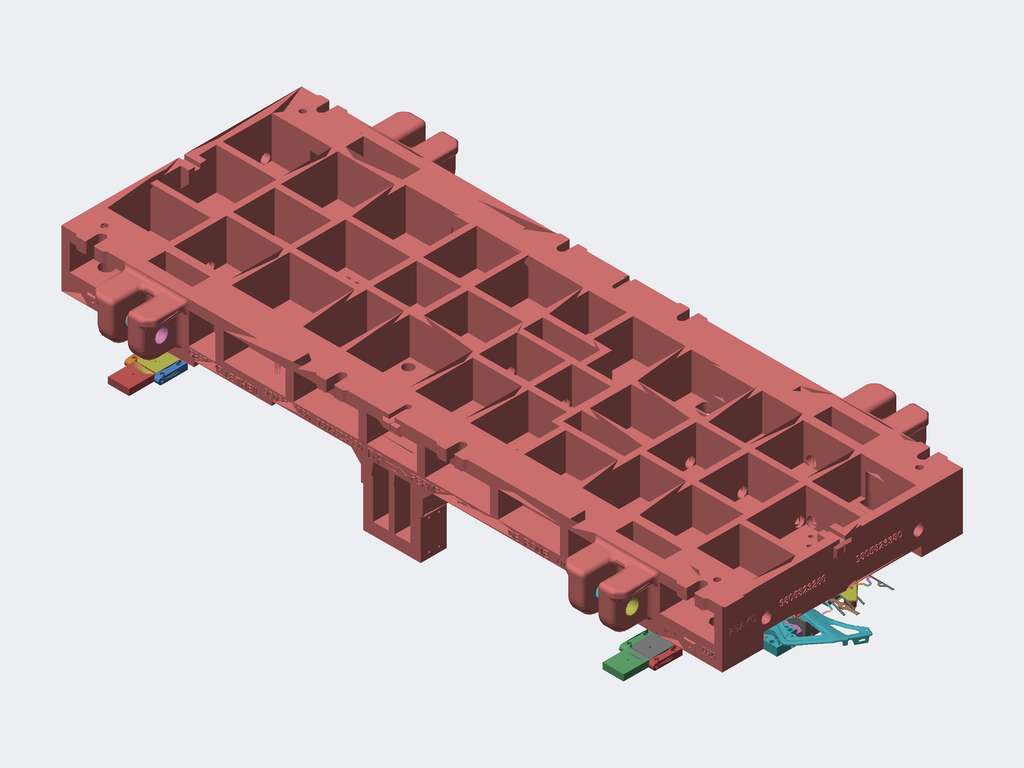Assembly | STEP file | 465 different items | 465 placed
Parts list (item | name | quantity | parent item | size | volume), first 255 of 465 items:
1 | gslz 2016.10.28-13_id1862_x_t | x1 | in gslz 2016.10.28-13_x_t | 105 x 145.1 x 30 mm | 436893 mm3
2 | gslz 2016.10.28-13_id1858_x_t | x1 | in gslz 2016.10.28-13_x_t | 105 x 145.1 x 30 mm | 436893 mm3
3 | gslz 2016.10.28-13_id1854_x_t | x1 | in gslz 2016.10.28-13_x_t | 105 x 145.1 x 30 mm | 436893 mm3
4 | gslz 2016.10.28-13_id1850_x_t | x1 | in gslz 2016.10.28-13_x_t | 105 x 145.1 x 30 mm | 436893 mm3
5 | gslz 2016.10.28-13_id1846_x_t | x1 | in gslz 2016.10.28-13_x_t | 33 x 145.1 x 30 mm | 128184 mm3
6 | gslz 2016.10.28-13_id1842_x_t | x1 | in gslz 2016.10.28-13_x_t | 105 x 145.1 x 30 mm | 436893 mm3
7 | gslz 2016.10.28-13_id1838_x_t | x1 | in gslz 2016.10.28-13_x_t | 105 x 145.1 x 30 mm | 436893 mm3
8 | gslz 2016.10.28-13_id1834_x_t | x1 | in gslz 2016.10.28-13_x_t | 105 x 145.1 x 30 mm | 436893 mm3
9 | gslz 2016.10.28-13_id1830_x_t | x1 | in gslz 2016.10.28-13_x_t | 105 x 145.1 x 30 mm | 436893 mm3
10 | gslz 2016.10.28-13_id1826_x_t | x1 | in gslz 2016.10.28-13_x_t | 23.336 x 25.084 x 18 mm | 4338 mm3
11 | gslz 2016.10.28-13_id1822_x_t | x1 | in gslz 2016.10.28-13_x_t | 23.336 x 25.084 x 18 mm | 4338 mm3
12 | gslz 2016.10.28-13_id1818_x_t | x1 | in gslz 2016.10.28-13_x_t | 78.589 x 55.064 x 12 mm | 30432 mm3
13 | gslz 2016.10.28-13_id1814_x_t | x1 | in gslz 2016.10.28-13_x_t | 79.537 x 58.997 x 10 mm | 15532 mm3
14 | gslz 2016.10.28-13_id1810_x_t | x1 | in gslz 2016.10.28-13_x_t | 101.812 x 70.347 x 10 mm | 22218 mm3
15 | gslz 2016.10.28-13_id1806_x_t | x1 | in gslz 2016.10.28-13_x_t | 101.812 x 70.347 x 10 mm | 22218 mm3
16 | gslz 2016.10.28-13_id1802_x_t | x1 | in gslz 2016.10.28-13_x_t | 30.396 x 23.404 x 12 mm | 3167 mm3
17 | gslz 2016.10.28-13_id1798_x_t | x1 | in gslz 2016.10.28-13_x_t | 30.396 x 23.404 x 12 mm | 3167 mm3
18 | gslz 2016.10.28-13_id1794_x_t | x1 | in gslz 2016.10.28-13_x_t | 48.801 x 30.009 x 15 mm | 3814 mm3
19 | gslz 2016.10.28-13_id1790_x_t | x1 | in gslz 2016.10.28-13_x_t | 48.801 x 30.009 x 15 mm | 3814 mm3
20 | gslz 2016.10.28-13_id1786_x_t | x1 | in gslz 2016.10.28-13_x_t | 29.214 x 38.304 x 56 mm | 22057 mm3
21 | gslz 2016.10.28-13_id1782_x_t | x1 | in gslz 2016.10.28-13_x_t | 37.214 x 54.544 x 22 mm | 10797 mm3
22 | gslz 2016.10.28-13_id1778_x_t | x1 | in gslz 2016.10.28-13_x_t | 41.743 x 29.62 x 14.53 mm | 4507 mm3
23 | gslz 2016.10.28-13_id1774_x_t | x1 | in gslz 2016.10.28-13_x_t | 102.493 x 71.684 x 27.5 mm | 56764 mm3
24 | gslz 2016.10.28-13_id1770_x_t | x1 | in gslz 2016.10.28-13_x_t | 102.493 x 71.684 x 27.5 mm | 56764 mm3
25 | gslz 2016.10.28-13_id1766_x_t | x1 | in gslz 2016.10.28-13_x_t | 159.469 x 183.505 x 86.5 mm | 557397 mm3
26 | gslz 2016.10.28-13_id1762_x_t | x1 | in gslz 2016.10.28-13_x_t | - | -
27 | 9805823280.1BPIECE_SOLIDE_FINALE_id1758_x_t | x1 | in gslz 2016.10.28-13_x_t | 12.56 x 23.021 x 8.234 mm | 240.263 mm3
28 | 1_id1754_x_t | x1 | in gslz 2016.10.28-13_x_t | 45.134 x 45.134 x 19 mm | 11498 mm3
29 | 1_id1750_x_t | x1 | in gslz 2016.10.28-13_x_t | 52.205 x 48.73 x 19 mm | 13276 mm3
30 | gslz 2016.10.28-13_id1746_x_t | x1 | in gslz 2016.10.28-13_x_t | 17 x 26 x 49 mm | 16052 mm3
31 | gslz 2016.10.28-13_id1742_x_t | x1 | in gslz 2016.10.28-13_x_t | 36 x 68 x 6 mm | 13161 mm3
32 | gslz 2016.10.28-13_id1738_x_t | x1 | in gslz 2016.10.28-13_x_t | 36 x 73 x 6 mm | 12869 mm3
33 | gslz 2016.10.28-13_id1734_x_t | x1 | in gslz 2016.10.28-13_x_t | 36 x 68 x 6 mm | 13161 mm3
34 | gslz 2016.10.28-13_id1730_x_t | x1 | in gslz 2016.10.28-13_x_t | 36 x 73 x 6 mm | 12869 mm3
35 | gslz 2016.10.28-13_id1726_x_t | x1 | in gslz 2016.10.28-13_x_t | 45 x 83 x 6 mm | 19739 mm3
36 | gslz 2016.10.28-13_id1722_x_t | x1 | in gslz 2016.10.28-13_x_t | 45 x 88 x 6 mm | 19661 mm3
37 | gslz 2016.10.28-13_id1718_x_t | x1 | in gslz 2016.10.28-13_x_t | 65 x 58 x 6 mm | 19127 mm3
38 | gslz 2016.10.28-13_id1714_x_t | x1 | in gslz 2016.10.28-13_x_t | 65 x 63 x 6 mm | 18675 mm3
39 | gslz 2016.10.28-13_id1710_x_t | x1 | in gslz 2016.10.28-13_x_t | 17 x 25 x 49 mm | 15358 mm3
40 | gslz 2016.10.28-13_id1706_x_t | x1 | in gslz 2016.10.28-13_x_t | 87.307 x 59.069 x 5 mm | 20118 mm3
41 | gslz 2016.10.28-13_id1702_x_t | x1 | in gslz 2016.10.28-13_x_t | 88.351 x 60.113 x 25 mm | 76522 mm3
42 | gslz 2016.10.28-13_id1698_x_t | x1 | in gslz 2016.10.28-13_x_t | 308.791 x 150.802 x 82.369 mm | 1185537 mm3
43 | gslz 2016.10.28-13_id1694_x_t | x1 | in gslz 2016.10.28-13_x_t | 72 x 35 x 5 mm | 11553 mm3
44 | gslz 2016.10.28-13_id1690_x_t | x1 | in gslz 2016.10.28-13_x_t | 69.906 x 50.319 x 5 mm | 9493 mm3
45 | gslz 2016.10.28-13_id1686_x_t | x1 | in gslz 2016.10.28-13_x_t | 64.831 x 66.474 x 5 mm | 11193 mm3
46 | gslz 2016.10.28-13_id1682_x_t | x1 | in gslz 2016.10.28-13_x_t | 67.358 x 53.937 x 5 mm | 9493 mm3
47 | gslz 2016.10.28-13_id1678_x_t | x1 | in gslz 2016.10.28-13_x_t | 73 x 36 x 26 mm | 45297 mm3
48 | gslz 2016.10.28-13_id1674_x_t | x1 | in gslz 2016.10.28-13_x_t | 70.882 x 51.053 x 36 mm | 51884 mm3
49 | gslz 2016.10.28-13_id1670_x_t | x1 | in gslz 2016.10.28-13_x_t | 68.435 x 55.014 x 26 mm | 39925 mm3
50 | gslz 2016.10.28-13_id1666_x_t | x1 | in gslz 2016.10.28-13_x_t | 65.839 x 67.482 x 31 mm | 54828 mm3
51 | gslz 2016.10.28-13_id1662_x_t | x1 | in gslz 2016.10.28-13_x_t | 29.227 x 19.541 x 70.5 mm | 21986 mm3
52 | gslz 2016.10.28-13_id1658_x_t | x1 | in gslz 2016.10.28-13_x_t | 32.149 x 22.13 x 70 mm | 26166 mm3
53 | gslz 2016.10.28-13_id1654_x_t | x1 | in gslz 2016.10.28-13_x_t | 46 x 23 x 10 mm | 9308 mm3
54 | gslz 2016.10.28-13_id1650_x_t | x1 | in gslz 2016.10.28-13_x_t | 43.888 x 21.981 x 24.856 mm | 5888 mm3
55 | gslz 2016.10.28-13_id1646_x_t | x1 | in gslz 2016.10.28-13_x_t | 105 x 520 x 15 mm | 667550 mm3
56 | gslz 2016.10.28-13_id1642_x_t | x1 | in gslz 2016.10.28-13_x_t | 180 x 40 x 32 mm | 197761 mm3
57 | gslz 2016.10.28-13_id1638_x_t | x1 | in gslz 2016.10.28-13_x_t | 110 x 90.115 x 79.8 mm | 541473 mm3
58 | gslz 2016.10.28-13_id1634_x_t | x1 | in gslz 2016.10.28-13_x_t | 39.238 x 33.552 x 28.984 mm | 15189 mm3
59 | gslz 2016.10.28-13_id1630_x_t | x1 | in gslz 2016.10.28-13_x_t | 158 x 98 x 72.916 mm | 768512 mm3
60 | gslz 2016.10.28-13_id1626_x_t | x1 | in gslz 2016.10.28-13_x_t | 42.516 x 42.404 x 26.831 mm | 17674 mm3
61 | gslz 2016.10.28-13_id1622_x_t | x1 | in gslz 2016.10.28-13_x_t | 17 x 20 x 49 mm | 11659 mm3
62 | gslz 2016.10.28-13_id1618_x_t | x1 | in gslz 2016.10.28-13_x_t | 57 x 88 x 63 mm | 168012 mm3
63 | 9805823380.1BPIECE_SOLIDE_FINALE_id1614_x_t | x1 | in gslz 2016.10.28-13_x_t | 252.902 x 148 x 67.965 mm | 1153711 mm3
64 | gslz 2016.10.28-13_id1610_x_t | x1 | in gslz 2016.10.28-13_x_t | 85 x 71 x 16 mm | 81626 mm3
65 | gslz 2016.10.28-13_id1606_x_t | x1 | in gslz 2016.10.28-13_x_t | 85 x 71 x 32 mm | 153487 mm3
66 | gslz 2016.10.28-13_id1602_x_t | x1 | in gslz 2016.10.28-13_x_t | 85 x 28 x 6 mm | 11529 mm3
67 | gslz 2016.10.28-13_id1598_x_t | x1 | in gslz 2016.10.28-13_x_t | 85 x 33 x 6 mm | 12707 mm3
68 | gslz 2016.10.28-13_id1594_x_t | x1 | in gslz 2016.10.28-13_x_t | 135 x 28 x 6 mm | 19929 mm3
69 | gslz 2016.10.28-13_id1590_x_t | x1 | in gslz 2016.10.28-13_x_t | 135 x 33 x 6 mm | 22607 mm3
70 | gslz 2016.10.28-13_id1586_x_t | x1 | in gslz 2016.10.28-13_x_t | 76 x 28 x 6 mm | 11241 mm3
71 | gslz 2016.10.28-13_id1582_x_t | x1 | in gslz 2016.10.28-13_x_t | 76 x 33 x 6 mm | 12149 mm3
72 | gslz 2016.10.28-13_id1578_x_t | x1 | in gslz 2016.10.28-13_x_t | 150 x 28 x 6 mm | 23673 mm3
73 | gslz 2016.10.28-13_id1574_x_t | x1 | in gslz 2016.10.28-13_x_t | 150 x 33 x 6 mm | 26801 mm3
74 | gslz 2016.10.28-13_id1570_x_t | x1 | in gslz 2016.10.28-13_x_t | 730 x 120 x 32 mm | 1766877 mm3
75 | gslz 2016.10.28-13_id1566_x_t | x1 | in gslz 2016.10.28-13_x_t | 810 x 120 x 32 mm | 2005033 mm3
76 | gslz 2016.10.28-13_id1562_x_t | x1 | in gslz 2016.10.28-13_x_t | 27.764 x 27.764 x 29.737 mm | 5874 mm3
77 | gslz 2016.10.28-13_id1558_x_t | x1 | in gslz 2016.10.28-13_x_t | 124.158 x 124.158 x 39.786 mm | 35566 mm3
78 | gslz 2016.10.28-13_id1554_x_t | x1 | in gslz 2016.10.28-13_x_t | 124.158 x 124.158 x 39.786 mm | 35566 mm3
79 | gslz 2016.10.28-13_id1550_x_t | x1 | in gslz 2016.10.28-13_x_t | 124.501 x 121.928 x 56.838 mm | 87407 mm3
80 | gslz 2016.10.28-13_id1546_x_t | x1 | in gslz 2016.10.28-13_x_t | 121.928 x 124.501 x 56.838 mm | 87407 mm3
81 | gslz 2016.10.28-13_id1542_x_t | x1 | in gslz 2016.10.28-13_x_t | 234.759 x 255.973 x 69 mm | 1431737 mm3
82 | gslz 2016.10.28-13_id1538_x_t | x1 | in gslz 2016.10.28-13_x_t | 27.148 x 27.148 x 16.361 mm | 2153 mm3
83 | gslz 2016.10.28-13_id1534_x_t | x1 | in gslz 2016.10.28-13_x_t | 27.622 x 23.712 x 48.072 mm | 19234 mm3
84 | gslz 2016.10.28-13_id1530_x_t | x1 | in gslz 2016.10.28-13_x_t | 123 x 53 x 40 mm | 161709 mm3
85 | gslz 2016.10.28-13_id1526_x_t | x1 | in gslz 2016.10.28-13_x_t | 45 x 30 x 75.242 mm | 77989 mm3
86 | gslz 2016.10.28-13_id1522_x_t | x1 | in gslz 2016.10.28-13_x_t | - | 122117 mm3
87 | gslz 2016.10.28-13_id1518_x_t | x1 | in gslz 2016.10.28-13_x_t | 29.762 x 31.599 x 21.259 mm | 4382 mm3
88 | gslz 2016.10.28-13_id1514_x_t | x1 | in gslz 2016.10.28-13_x_t | 198.697 x 124.174 x 92.051 mm | 929934 mm3
89 | gslz 2016.10.28-13_id1510_x_t | x1 | in gslz 2016.10.28-13_x_t | 60.365 x 38.336 x 39 mm | 43186 mm3
90 | gslz 2016.10.28-13_id1506_x_t | x1 | in gslz 2016.10.28-13_x_t | 44.234 x 36.078 x 44 mm | 40757 mm3
91 | gslz 2016.10.28-13_id1502_x_t | x1 | in gslz 2016.10.28-13_x_t | - | -
92 | gslz 2016.10.28-13_id1498_x_t | x1 | in gslz 2016.10.28-13_x_t | - | -
93 | gslz 2016.10.28-13_id1494_x_t | x1 | in gslz 2016.10.28-13_x_t | - | -
94 | gslz 2016.10.28-13_id1490_x_t | x1 | in gslz 2016.10.28-13_x_t | - | -
95 | gslz 2016.10.28-13_id1486_x_t | x1 | in gslz 2016.10.28-13_x_t | - | -
96 | gslz 2016.10.28-13_id1482_x_t | x1 | in gslz 2016.10.28-13_x_t | 48.587 x 48.391 x 29.021 mm | 10993 mm3
97 | gslz 2016.10.28-13_id1478_x_t | x1 | in gslz 2016.10.28-13_x_t | 25.456 x 25.456 x 27 mm | 6738 mm3
98 | gslz 2016.10.28-13_id1474_x_t | x1 | in gslz 2016.10.28-13_x_t | 22.953 x 24.888 x 27 mm | 6892 mm3
99 | gslz 2016.10.28-13_id1470_x_t | x1 | in gslz 2016.10.28-13_x_t | 66.885 x 98.566 x 27.5 mm | 53451 mm3
100 | gslz 2016.10.28-13_id1466_x_t | x1 | in gslz 2016.10.28-13_x_t | 67.638 x 102.464 x 10 mm | 22218 mm3
101 | gslz 2016.10.28-13_id1462_x_t | x1 | in gslz 2016.10.28-13_x_t | 67.638 x 102.464 x 10 mm | 22218 mm3
102 | gslz 2016.10.28-13_id1458_x_t | x1 | in gslz 2016.10.28-13_x_t | 66.885 x 98.566 x 27.5 mm | 53451 mm3
103 | gslz 2016.10.28-13_id1454_x_t | x1 | in gslz 2016.10.28-13_x_t | 81.802 x 53.748 x 52 mm | 84086 mm3
104 | gslz 2016.10.28-13_id1450_x_t | x1 | in gslz 2016.10.28-13_x_t | 160.575 x 107.178 x 72.851 mm | 541622 mm3
105 | gslz 2016.10.28-13_id1446_x_t | x1 | in gslz 2016.10.28-13_x_t | 9.039 x 11.595 x 1.56 mm | 84.551 mm3
106 | gslz 2016.10.28-13_id1442_x_t | x1 | in gslz 2016.10.28-13_x_t | - | -
107 | gslz 2016.10.28-13_id1438_x_t | x1 | in gslz 2016.10.28-13_x_t | - | -
108 | gslz 2016.10.28-13_id1434_x_t | x1 | in gslz 2016.10.28-13_x_t | - | -
109 | gslz 2016.10.28-13_id1430_x_t | x1 | in gslz 2016.10.28-13_x_t | - | -
110 | gslz 2016.10.28-13_id1426_x_t | x1 | in gslz 2016.10.28-13_x_t | - | -
111 | gslz 2016.10.28-13_id1422_x_t | x1 | in gslz 2016.10.28-13_x_t | 96.313 x 39.023 x 74.019 mm | 168785 mm3
112 | gslz 2016.10.28-13_id1418_x_t | x1 | in gslz 2016.10.28-13_x_t | 415 x 296 x 77.793 mm | 6493168 mm3
113 | gslz 2016.10.28-13_id1414_x_t | x1 | in gslz 2016.10.28-13_x_t | - | -
114 | gslz 2016.10.28-13_id1410_x_t | x1 | in gslz 2016.10.28-13_x_t | - | -
115 | gslz 2016.10.28-13_id1406_x_t | x1 | in gslz 2016.10.28-13_x_t | - | -
116 | gslz 2016.10.28-13_id1402_x_t | x1 | in gslz 2016.10.28-13_x_t | 90.51 x 90.51 x 10 mm | 22218 mm3
117 | gslz 2016.10.28-13_id1398_x_t | x1 | in gslz 2016.10.28-13_x_t | 90.51 x 90.51 x 10 mm | 22218 mm3
118 | gslz 2016.10.28-13_id1394_x_t | x1 | in gslz 2016.10.28-13_x_t | 50.205 x 48.083 x 16 mm | 10037 mm3
119 | gslz 2016.10.28-13_id1390_x_t | x1 | in gslz 2016.10.28-13_x_t | 37.477 x 39.598 x 16 mm | 7157 mm3
120 | gslz 2016.10.28-13_id1386_x_t | x1 | in gslz 2016.10.28-13_x_t | 91.57 x 91.57 x 27.5 mm | 56764 mm3
121 | gslz 2016.10.28-13_id1382_x_t | x1 | in gslz 2016.10.28-13_x_t | 43.55 x 43.55 x 48.008 mm | 15438 mm3
122 | gslz 2016.10.28-13_id1378_x_t | x1 | in gslz 2016.10.28-13_x_t | 91.57 x 91.57 x 27.5 mm | 56764 mm3
123 | gslz 2016.10.28-13_id1374_x_t | x1 | in gslz 2016.10.28-13_x_t | 48.79 x 48.79 x 60 mm | 42680 mm3
124 | gslz 2016.10.28-13_id1370_x_t | x1 | in gslz 2016.10.28-13_x_t | 46.5 x 32.8 x 73 mm | 100113 mm3
125 | gslz 2016.10.28-13_id1366_x_t | x1 | in gslz 2016.10.28-13_x_t | 51.5 x 24.8 x 73 mm | 72067 mm3
126 | gslz 2016.10.28-13_id1362_x_t | x1 | in gslz 2016.10.28-13_x_t | - | -
127 | gslz 2016.10.28-13_id1358_x_t | x1 | in gslz 2016.10.28-13_x_t | 114 x 26.5 x 48 mm | 106202 mm3
128 | gslz 2016.10.28-13_id1354_x_t | x1 | in gslz 2016.10.28-13_x_t | 73.861 x 76.347 x 57.728 mm | 171700 mm3
129 | gslz 2016.10.28-13_id1350_x_t | x1 | in gslz 2016.10.28-13_x_t | 339.5 x 207 x 81.123 mm | 2655764 mm3
130 | gslz 2016.10.28-13_id1346_x_t | x1 | in gslz 2016.10.28-13_x_t | - | -
131 | gslz 2016.10.28-13_id1342_x_t | x1 | in gslz 2016.10.28-13_x_t | 347 x 40 x 48 mm | 605773 mm3
132 | gslz 2016.10.28-13_id1338_x_t | x1 | in gslz 2016.10.28-13_x_t | 348 x 40 x 48 mm | 621204 mm3
133 | gslz 2016.10.28-13_id1334_x_t | x1 | in gslz 2016.10.28-13_x_t | 95 x 65 x 32 mm | 157873 mm3
134 | gslz 2016.10.28-13_id1330_x_t | x1 | in gslz 2016.10.28-13_x_t | 12.175 x 9.008 x 2.356 mm | 107.013 mm3
135 | gslz 2016.10.28-13_id1326_x_t | x1 | in gslz 2016.10.28-13_x_t | 8.284 x 8.42 x 2.147 mm | 67.466 mm3
136 | FINAL_SOLID_PART_id1322_x_t | x1 | in gslz 2016.10.28-13_x_t | - | -
137 | gslz 2016.10.28-13_id1318_x_t | x1 | in gslz 2016.10.28-13_x_t | 117.473 x 52.739 x 8.208 mm | 4131 mm3
138 | gslz 2016.10.28-13_id1314_x_t | x1 | in gslz 2016.10.28-13_x_t | - | -
139 | gslz 2016.10.28-13_id1310_x_t | x1 | in gslz 2016.10.28-13_x_t | - | -
140 | gslz 2016.10.28-13_id1306_x_t | x1 | in gslz 2016.10.28-13_x_t | - | -
141 | gslz 2016.10.28-13_id1302_x_t | x1 | in gslz 2016.10.28-13_x_t | - | -
142 | gslz 2016.10.28-13_id1298_x_t | x1 | in gslz 2016.10.28-13_x_t | - | -
143 | gslz 2016.10.28-13_id1294_x_t | x1 | in gslz 2016.10.28-13_x_t | - | -
144 | gslz 2016.10.28-13_id1290_x_t | x1 | in gslz 2016.10.28-13_x_t | - | -
145 | gslz 2016.10.28-13_id1286_x_t | x1 | in gslz 2016.10.28-13_x_t | - | -
146 | gslz 2016.10.28-13_id1282_x_t | x1 | in gslz 2016.10.28-13_x_t | - | -
147 | gslz 2016.10.28-13_id1278_x_t | x1 | in gslz 2016.10.28-13_x_t | - | -
148 | gslz 2016.10.28-13_id1274_x_t | x1 | in gslz 2016.10.28-13_x_t | - | -
149 | gslz 2016.10.28-13_id1270_x_t | x1 | in gslz 2016.10.28-13_x_t | - | -
150 | gslz 2016.10.28-13_id1266_x_t | x1 | in gslz 2016.10.28-13_x_t | - | -
151 | gslz 2016.10.28-13_id1262_x_t | x1 | in gslz 2016.10.28-13_x_t | - | -
152 | gslz 2016.10.28-13_id1258_x_t | x1 | in gslz 2016.10.28-13_x_t | - | 526.34 mm3
153 | gslz 2016.10.28-13_id1254_x_t | x1 | in gslz 2016.10.28-13_x_t | 50.336 x 46.733 x 12.552 mm | 985.225 mm3
154 | gslz 2016.10.28-13_id1250_x_t | x1 | in gslz 2016.10.28-13_x_t | 40.597 x 86.839 x 25.215 mm | 1239 mm3
155 | gslz 2016.10.28-13_id1246_x_t | x1 | in gslz 2016.10.28-13_x_t | - | -
156 | gslz 2016.10.28-13_id1242_x_t | x1 | in gslz 2016.10.28-13_x_t | - | -
157 | gslz 2016.10.28-13_id1238_x_t | x1 | in gslz 2016.10.28-13_x_t | - | -
158 | gslz 2016.10.28-13_id1234_x_t | x1 | in gslz 2016.10.28-13_x_t | - | -
159 | gslz 2016.10.28-13_id1230_x_t | x1 | in gslz 2016.10.28-13_x_t | 63.363 x 44.787 x 14.43 mm | 927.066 mm3
160 | gslz 2016.10.28-13_id1226_x_t | x1 | in gslz 2016.10.28-13_x_t | - | 746.006 mm3
161 | gslz 2016.10.28-13_id1222_x_t | x1 | in gslz 2016.10.28-13_x_t | - | 746.006 mm3
162 | gslz 2016.10.28-13_id1218_x_t | x1 | in gslz 2016.10.28-13_x_t | 63.363 x 44.787 x 14.43 mm | 927.564 mm3
163 | gslz 2016.10.28-13_id1214_x_t | x1 | in gslz 2016.10.28-13_x_t | 335 x 25.5 x 4 mm | 5252 mm3
164 | gslz 2016.10.28-13_id1210_x_t | x1 | in gslz 2016.10.28-13_x_t | 335 x 25.5 x 4 mm | 5252 mm3
165 | gslz 2016.10.28-13_id1206_x_t | x1 | in gslz 2016.10.28-13_x_t | 335 x 25.5 x 4 mm | 5252 mm3
166 | gslz 2016.10.28-13_id1202_x_t | x1 | in gslz 2016.10.28-13_x_t | 335 x 25.5 x 4 mm | 5252 mm3
167 | gslz 2016.10.28-13_id1198_x_t | x1 | in gslz 2016.10.28-13_x_t | 235 x 25.5 x 4 mm | 3805 mm3
168 | FINAL_SOLID_PART_id1194_x_t | x1 | in gslz 2016.10.28-13_x_t | - | -
169 | FINAL_SOLID_PART_id1190_x_t | x1 | in gslz 2016.10.28-13_x_t | - | -
170 | gslz 2016.10.28-13_id1186_x_t | x1 | in gslz 2016.10.28-13_x_t | - | -
171 | gslz 2016.10.28-13_id1182_x_t | x1 | in gslz 2016.10.28-13_x_t | - | -
172 | gslz 2016.10.28-13_id1178_x_t | x1 | in gslz 2016.10.28-13_x_t | 12.2 x 12.2 x 1.25 mm | 146.123 mm3
173 | gslz 2016.10.28-13_id1174_x_t | x1 | in gslz 2016.10.28-13_x_t | 40 x 20 x 1.25 mm | 719.671 mm3
174 | gslz 2016.10.28-13_id1170_x_t | x1 | in gslz 2016.10.28-13_x_t | 6.934 x 8.042 x 1.25 mm | 0.6004 mm3
175 | gslz 2016.10.28-13_id1166_x_t | x1 | in gslz 2016.10.28-13_x_t | 216.271 x 15 x 1.25 mm | 4055 mm3
176 | gslz 2016.10.28-13_id1162_x_t | x1 | in gslz 2016.10.28-13_x_t | 8.449 x 8.449 x 1.25 mm | 67.248 mm3
177 | gslz 2016.10.28-13_id1158_x_t | x1 | in gslz 2016.10.28-13_x_t | 12.076 x 9.187 x 1.25 mm | 107.013 mm3
178 | gslz 2016.10.28-13_id1154_x_t | x1 | in gslz 2016.10.28-13_x_t | 8.449 x 8.449 x 1.25 mm | 67.248 mm3
179 | gslz 2016.10.28-13_id1150_x_t | x1 | in gslz 2016.10.28-13_x_t | 12.076 x 9.187 x 1.25 mm | 107.013 mm3
180 | gslz 2016.10.28-13_id1146_x_t | x1 | in gslz 2016.10.28-13_x_t | 159.005 x 29 x 8 mm | 3787 mm3
181 | gslz 2016.10.28-13_id1142_x_t | x1 | in gslz 2016.10.28-13_x_t | 335 x 29 x 8 mm | 7083 mm3
182 | gslz 2016.10.28-13_id1138_x_t | x1 | in gslz 2016.10.28-13_x_t | 335 x 29 x 8 mm | 7083 mm3
183 | gslz 2016.10.28-13_id1134_x_t | x1 | in gslz 2016.10.28-13_x_t | 335 x 29 x 8 mm | 7083 mm3
184 | gslz 2016.10.28-13_id1130_x_t | x1 | in gslz 2016.10.28-13_x_t | 335 x 29 x 8 mm | 7083 mm3
185 | 9805823380.1BPIECE_SOLIDE_FINALE_id1126_x_t | x1 | in gslz 2016.10.28-13_x_t | 308.018 x 147.7 x 55.936 mm | 34010 mm3
186 | gslz 2016.10.28-13_id1122_x_t | x1 | in gslz 2016.10.28-13_x_t | 139 x 100 x 32 mm | 383578 mm3
187 | gslz 2016.10.28-13_id1118_x_t | x1 | in gslz 2016.10.28-13_x_t | 335 x 29 x 8 mm | 7083 mm3
188 | gslz 2016.10.28-13_id1114_x_t | x1 | in gslz 2016.10.28-13_x_t | 6.882 x 6.913 x 8.538 mm | 70.931 mm3
189 | gslz 2016.10.28-13_id1110_x_t | x1 | in gslz 2016.10.28-13_x_t | 9.039 x 11.595 x 1.56 mm | 84.551 mm3
190 | gslz 2016.10.28-13_id1106_x_t | x1 | in gslz 2016.10.28-13_x_t | 8.332 x 8.174 x 3.149 mm | 67.466 mm3
191 | gslz 2016.10.28-13_id1102_x_t | x1 | in gslz 2016.10.28-13_x_t | 12.193 x 8.988 x 2.236 mm | 107.013 mm3
192 | gslz 2016.10.28-13_id1098_x_t | x1 | in gslz 2016.10.28-13_x_t | 117.479 x 52.908 x 8.668 mm | 4131 mm3
193 | gslz 2016.10.28-13_id1094_x_t | x1 | in gslz 2016.10.28-13_x_t | 18.724 x 18.722 x 8.278 mm | 240.264 mm3
194 | gslz 2016.10.28-13_id1090_x_t | x1 | in gslz 2016.10.28-13_x_t | 18.265 x 18.776 x 11.14 mm | 240.265 mm3
195 | gslz 2016.10.28-13_id1086_x_t | x1 | in gslz 2016.10.28-13_x_t | 6.311 x 6.312 x 2.41 mm | 37.737 mm3
196 | gslz 2016.10.28-13_id1082_x_t | x1 | in gslz 2016.10.28-13_x_t | 11.029 x 10.034 x 2.548 mm | 84.369 mm3
197 | gslz 2016.10.28-13_id1078_x_t | x1 | in gslz 2016.10.28-13_x_t | 8.197 x 8.356 x 2.88 mm | 67.248 mm3
198 | gslz 2016.10.28-13_id1074_x_t | x1 | in gslz 2016.10.28-13_x_t | 12.113 x 9.24 x 3.468 mm | 107.013 mm3
199 | gslz 2016.10.28-13_id1070_x_t | x1 | in gslz 2016.10.28-13_x_t | 10.965 x 9.974 x 2.304 mm | 84.369 mm3
200 | gslz 2016.10.28-13_id1066_x_t | x1 | in gslz 2016.10.28-13_x_t | 6.254 x 6.275 x 1.796 mm | 37.737 mm3
201 | gslz 2016.10.28-13_id1062_x_t | x1 | in gslz 2016.10.28-13_x_t | 6.872 x 6.937 x 8.903 mm | 72.493 mm3
202 | gslz 2016.10.28-13_id1058_x_t | x1 | in gslz 2016.10.28-13_x_t | 12.113 x 9.24 x 3.468 mm | 107.013 mm3
203 | gslz 2016.10.28-13_id1054_x_t | x1 | in gslz 2016.10.28-13_x_t | 6.254 x 6.275 x 1.796 mm | 37.737 mm3
204 | gslz 2016.10.28-13_id1050_x_t | x1 | in gslz 2016.10.28-13_x_t | 10.965 x 9.974 x 2.304 mm | 84.369 mm3
205 | gslz 2016.10.28-13_id1046_x_t | x1 | in gslz 2016.10.28-13_x_t | 8.197 x 8.356 x 2.88 mm | 67.248 mm3
206 | 9805823380.1BPIECE_SOLIDE_FINALE_id1042_x_t | x1 | in gslz 2016.10.28-13_x_t | 329.111 x 160.705 x 37.841 mm | 35454 mm3
207 | gslz 2016.10.28-13_id1038_x_t | x1 | in gslz 2016.10.28-13_x_t | 335 x 25.5 x 4 mm | 5252 mm3
208 | gslz 2016.10.28-13_id1034_x_t | x1 | in gslz 2016.10.28-13_x_t | 253.449 x 25.5 x 4 mm | 4072 mm3
209 | gslz 2016.10.28-13_id1030_x_t | x1 | in gslz 2016.10.28-13_x_t | 335 x 25.5 x 4 mm | 5252 mm3
210 | gslz 2016.10.28-13_id1026_x_t | x1 | in gslz 2016.10.28-13_x_t | 335 x 25.5 x 4 mm | 5252 mm3
211 | gslz 2016.10.28-13_id1022_x_t | x1 | in gslz 2016.10.28-13_x_t | 335 x 25.5 x 4 mm | 5252 mm3
212 | gslz 2016.10.28-13_id1018_x_t | x1 | in gslz 2016.10.28-13_x_t | 335 x 25.5 x 4 mm | 5252 mm3
213 | gslz 2016.10.28-13_id1014_x_t | x1 | in gslz 2016.10.28-13_x_t | 335 x 25.5 x 4 mm | 5252 mm3
214 | gslz 2016.10.28-13_id1010_x_t | x1 | in gslz 2016.10.28-13_x_t | 12.3 x 12.3 x 1.25 mm | 148.529 mm3
215 | gslz 2016.10.28-13_id1006_x_t | x1 | in gslz 2016.10.28-13_x_t | 12.3 x 12.3 x 1.25 mm | 148.529 mm3
216 | 9805823380.1BPIECE_SOLIDE_FINALE_id1002_x_t | x1 | in gslz 2016.10.28-13_x_t | 307.193 x 147.409 x 65.496 mm | 34010 mm3
217 | 9805823380.1BPIECE_SOLIDE_FINALE_id998_x_t | x1 | in gslz 2016.10.28-13_x_t | 307.193 x 147.409 x 65.496 mm | 34012 mm3
218 | gslz 2016.10.28-13_id994_x_t | x1 | in gslz 2016.10.28-13_x_t | 903 x 64 x 38 mm | 1224228 mm3
219 | gslz 2016.10.28-13_id990_x_t | x1 | in gslz 2016.10.28-13_x_t | 730 x 68 x 38 mm | 1131774 mm3
220 | gslz 2016.10.28-13_id986_x_t | x1 | in gslz 2016.10.28-13_x_t | 117.479 x 52.908 x 8.668 mm | 4131 mm3
221 | gslz 2016.10.28-13_id982_x_t | x1 | in gslz 2016.10.28-13_x_t | - | -
222 | FINAL_SOLID_PART_id978_x_t | x1 | in gslz 2016.10.28-13_x_t | - | -
223 | gslz 2016.10.28-13_id974_x_t | x1 | in gslz 2016.10.28-13_x_t | 335 x 29 x 8 mm | 7097 mm3
224 | gslz 2016.10.28-13_id970_x_t | x1 | in gslz 2016.10.28-13_x_t | 29.791 x 13 x 4 mm | 449.169 mm3
225 | gslz 2016.10.28-13_id966_x_t | x1 | in gslz 2016.10.28-13_x_t | 255.209 x 9 x 4 mm | 3693 mm3
226 | gslz 2016.10.28-13_id962_x_t | x1 | in gslz 2016.10.28-13_x_t | 60 x 25.5 x 4 mm | 1272 mm3
227 | gslz 2016.10.28-13_id958_x_t | x1 | in gslz 2016.10.28-13_x_t | 436.271 x 29.5 x 4 mm | 6895 mm3
228 | gslz 2016.10.28-13_id954_x_t | x1 | in gslz 2016.10.28-13_x_t | 8.945 x 8.722 x 12.3 mm | 358.338 mm3
229 | gslz 2016.10.28-13_id950_x_t | x1 | in gslz 2016.10.28-13_x_t | 8.945 x 8.722 x 12.3 mm | 357.729 mm3
230 | gslz 2016.10.28-13_id946_x_t | x1 | in gslz 2016.10.28-13_x_t | 8.945 x 8.722 x 12 mm | 357 mm3
231 | gslz 2016.10.28-13_id942_x_t | x1 | in gslz 2016.10.28-13_x_t | 5.723 x 9.158 x 12.3 mm | 358.338 mm3
232 | gslz 2016.10.28-13_id938_x_t | x1 | in gslz 2016.10.28-13_x_t | 5.723 x 9.158 x 12.3 mm | 358.512 mm3
233 | gslz 2016.10.28-13_id934_x_t | x1 | in gslz 2016.10.28-13_x_t | 8.945 x 8.722 x 12.3 mm | 358.512 mm3
234 | gslz 2016.10.28-13_id930_x_t | x1 | in gslz 2016.10.28-13_x_t | 5.723 x 9.158 x 12.3 mm | 358.483 mm3
235 | gslz 2016.10.28-13_id926_x_t | x1 | in gslz 2016.10.28-13_x_t | 5.723 x 9.158 x 12.3 mm | 357.729 mm3
236 | gslz 2016.10.28-13_id922_x_t | x1 | in gslz 2016.10.28-13_x_t | 8.945 x 8.722 x 12.3 mm | 357.729 mm3
237 | gslz 2016.10.28-13_id918_x_t | x1 | in gslz 2016.10.28-13_x_t | 8.945 x 8.722 x 12.3 mm | 358.206 mm3
238 | gslz 2016.10.28-13_id914_x_t | x1 | in gslz 2016.10.28-13_x_t | 8.945 x 8.722 x 12.3 mm | 358.471 mm3
239 | gslz 2016.10.28-13_id910_x_t | x1 | in gslz 2016.10.28-13_x_t | 5.723 x 9.158 x 12.3 mm | 358.44 mm3
240 | gslz 2016.10.28-13_id906_x_t | x1 | in gslz 2016.10.28-13_x_t | 8.945 x 8.722 x 12.3 mm | 358.244 mm3
241 | gslz 2016.10.28-13_id902_x_t | x1 | in gslz 2016.10.28-13_x_t | 5.723 x 9.158 x 12.3 mm | 357.729 mm3
242 | gslz 2016.10.28-13_id898_x_t | x1 | in gslz 2016.10.28-13_x_t | 8.945 x 8.722 x 12.3 mm | 358.206 mm3
243 | gslz 2016.10.28-13_id894_x_t | x1 | in gslz 2016.10.28-13_x_t | 5.723 x 9.158 x 12.3 mm | 358.344 mm3
244 | gslz 2016.10.28-13_id890_x_t | x1 | in gslz 2016.10.28-13_x_t | 8.945 x 8.722 x 12.3 mm | 358.44 mm3
245 | 9805823380.1BPIECE_SOLIDE_FINALE_id886_x_t | x1 | in gslz 2016.10.28-13_x_t | 308.018 x 147.7 x 55.936 mm | 34010 mm3
246 | gslz 2016.10.28-13_id882_x_t | x1 | in gslz 2016.10.28-13_x_t | 5.723 x 9.158 x 12.3 mm | 358.206 mm3
247 | gslz 2016.10.28-13_id878_x_t | x1 | in gslz 2016.10.28-13_x_t | 8.945 x 8.722 x 12 mm | 357 mm3
248 | gslz 2016.10.28-13_id874_x_t | x1 | in gslz 2016.10.28-13_x_t | 8.945 x 8.722 x 12 mm | 357 mm3
249 | gslz 2016.10.28-13_id870_x_t | x1 | in gslz 2016.10.28-13_x_t | 5.723 x 9.158 x 12.3 mm | 358.269 mm3
250 | gslz 2016.10.28-13_id866_x_t | x1 | in gslz 2016.10.28-13_x_t | 5.723 x 9.158 x 12.3 mm | 358.269 mm3
251 | gslz 2016.10.28-13_id862_x_t | x1 | in gslz 2016.10.28-13_x_t | 8.945 x 8.722 x 12.3 mm | 358.344 mm3
252 | gslz 2016.10.28-13_id858_x_t | x1 | in gslz 2016.10.28-13_x_t | 8.945 x 8.722 x 12.3 mm | 358.198 mm3
253 | 9805823280.1BPIECE_SOLIDE_FINALE_id854_x_t | x1 | in gslz 2016.10.28-13_x_t | 364.643 x 274.564 x 38.362 mm | 69005 mm3
254 | gslz 2016.10.28-13_id850_x_t | x1 | in gslz 2016.10.28-13_x_t | 5.723 x 9.158 x 12.3 mm | 358.483 mm3
255 | gslz 2016.10.28-13_id846_x_t | x1 | in gslz 2016.10.28-13_x_t | 8.945 x 8.722 x 12.3 mm | 358.512 mm3
Placements (level | parent | child | x y z in mm | rotation matrix by rows), first 175 of 465 lines:
1 | gslz 2016.10.28-13_x_t | gslz 2016.10.28-13_id1862_x_t | 0.0 0.0 0.0 | 1 0 0 0 1 0 0 0 1
1 | gslz 2016.10.28-13_x_t | gslz 2016.10.28-13_id1858_x_t | 0.0 0.0 0.0 | 1 0 0 0 1 0 0 0 1
1 | gslz 2016.10.28-13_x_t | gslz 2016.10.28-13_id1854_x_t | 0.0 0.0 0.0 | 1 0 0 0 1 0 0 0 1
1 | gslz 2016.10.28-13_x_t | gslz 2016.10.28-13_id1850_x_t | 0.0 0.0 0.0 | 1 0 0 0 1 0 0 0 1
1 | gslz 2016.10.28-13_x_t | gslz 2016.10.28-13_id1846_x_t | 0.0 0.0 0.0 | 1 0 0 0 1 0 0 0 1
1 | gslz 2016.10.28-13_x_t | gslz 2016.10.28-13_id1842_x_t | 0.0 0.0 0.0 | 1 0 0 0 1 0 0 0 1
1 | gslz 2016.10.28-13_x_t | gslz 2016.10.28-13_id1838_x_t | 0.0 0.0 0.0 | 1 0 0 0 1 0 0 0 1
1 | gslz 2016.10.28-13_x_t | gslz 2016.10.28-13_id1834_x_t | 0.0 0.0 0.0 | 1 0 0 0 1 0 0 0 1
1 | gslz 2016.10.28-13_x_t | gslz 2016.10.28-13_id1830_x_t | 0.0 0.0 0.0 | 1 0 0 0 1 0 0 0 1
1 | gslz 2016.10.28-13_x_t | gslz 2016.10.28-13_id1826_x_t | 0.0 0.0 0.0 | 1 0 0 0 1 0 0 0 1
1 | gslz 2016.10.28-13_x_t | gslz 2016.10.28-13_id1822_x_t | 0.0 0.0 0.0 | 1 0 0 0 1 0 0 0 1
1 | gslz 2016.10.28-13_x_t | gslz 2016.10.28-13_id1818_x_t | 0.0 0.0 0.0 | 1 0 0 0 1 0 0 0 1
1 | gslz 2016.10.28-13_x_t | gslz 2016.10.28-13_id1814_x_t | 0.0 0.0 0.0 | 1 0 0 0 1 0 0 0 1
1 | gslz 2016.10.28-13_x_t | gslz 2016.10.28-13_id1810_x_t | 0.0 0.0 0.0 | 1 0 0 0 1 0 0 0 1
1 | gslz 2016.10.28-13_x_t | gslz 2016.10.28-13_id1806_x_t | 0.0 0.0 0.0 | 1 0 0 0 1 0 0 0 1
1 | gslz 2016.10.28-13_x_t | gslz 2016.10.28-13_id1802_x_t | 0.0 0.0 0.0 | 1 0 0 0 1 0 0 0 1
1 | gslz 2016.10.28-13_x_t | gslz 2016.10.28-13_id1798_x_t | 0.0 0.0 0.0 | 1 0 0 0 1 0 0 0 1
1 | gslz 2016.10.28-13_x_t | gslz 2016.10.28-13_id1794_x_t | 0.0 0.0 0.0 | 1 0 0 0 1 0 0 0 1
1 | gslz 2016.10.28-13_x_t | gslz 2016.10.28-13_id1790_x_t | 0.0 0.0 0.0 | 1 0 0 0 1 0 0 0 1
1 | gslz 2016.10.28-13_x_t | gslz 2016.10.28-13_id1786_x_t | 0.0 0.0 0.0 | 1 0 0 0 1 0 0 0 1
1 | gslz 2016.10.28-13_x_t | gslz 2016.10.28-13_id1782_x_t | 0.0 0.0 0.0 | 1 0 0 0 1 0 0 0 1
1 | gslz 2016.10.28-13_x_t | gslz 2016.10.28-13_id1778_x_t | 0.0 0.0 0.0 | 1 0 0 0 1 0 0 0 1
1 | gslz 2016.10.28-13_x_t | gslz 2016.10.28-13_id1774_x_t | 0.0 0.0 0.0 | 1 0 0 0 1 0 0 0 1
1 | gslz 2016.10.28-13_x_t | gslz 2016.10.28-13_id1770_x_t | 0.0 0.0 0.0 | 1 0 0 0 1 0 0 0 1
1 | gslz 2016.10.28-13_x_t | gslz 2016.10.28-13_id1766_x_t | 0.0 0.0 0.0 | 1 0 0 0 1 0 0 0 1
1 | gslz 2016.10.28-13_x_t | gslz 2016.10.28-13_id1762_x_t | 0.0 0.0 0.0 | 1 0 0 0 1 0 0 0 1
1 | gslz 2016.10.28-13_x_t | 9805823280.1BPIECE_SOLIDE_FINALE_id1758_x_t | 0.0 0.0 0.0 | 1 0 0 0 1 0 0 0 1
1 | gslz 2016.10.28-13_x_t | 1_id1754_x_t | 0.0 0.0 0.0 | 1 0 0 0 1 0 0 0 1
1 | gslz 2016.10.28-13_x_t | 1_id1750_x_t | 0.0 0.0 0.0 | 1 0 0 0 1 0 0 0 1
1 | gslz 2016.10.28-13_x_t | gslz 2016.10.28-13_id1746_x_t | 0.0 0.0 0.0 | 1 0 0 0 1 0 0 0 1
1 | gslz 2016.10.28-13_x_t | gslz 2016.10.28-13_id1742_x_t | 0.0 0.0 0.0 | 1 0 0 0 1 0 0 0 1
1 | gslz 2016.10.28-13_x_t | gslz 2016.10.28-13_id1738_x_t | 0.0 0.0 0.0 | 1 0 0 0 1 0 0 0 1
1 | gslz 2016.10.28-13_x_t | gslz 2016.10.28-13_id1734_x_t | 0.0 0.0 0.0 | 1 0 0 0 1 0 0 0 1
1 | gslz 2016.10.28-13_x_t | gslz 2016.10.28-13_id1730_x_t | 0.0 0.0 0.0 | 1 0 0 0 1 0 0 0 1
1 | gslz 2016.10.28-13_x_t | gslz 2016.10.28-13_id1726_x_t | 0.0 0.0 0.0 | 1 0 0 0 1 0 0 0 1
1 | gslz 2016.10.28-13_x_t | gslz 2016.10.28-13_id1722_x_t | 0.0 0.0 0.0 | 1 0 0 0 1 0 0 0 1
1 | gslz 2016.10.28-13_x_t | gslz 2016.10.28-13_id1718_x_t | 0.0 0.0 0.0 | 1 0 0 0 1 0 0 0 1
1 | gslz 2016.10.28-13_x_t | gslz 2016.10.28-13_id1714_x_t | 0.0 0.0 0.0 | 1 0 0 0 1 0 0 0 1
1 | gslz 2016.10.28-13_x_t | gslz 2016.10.28-13_id1710_x_t | 0.0 0.0 0.0 | 1 0 0 0 1 0 0 0 1
1 | gslz 2016.10.28-13_x_t | gslz 2016.10.28-13_id1706_x_t | 0.0 0.0 0.0 | 1 0 0 0 1 0 0 0 1
1 | gslz 2016.10.28-13_x_t | gslz 2016.10.28-13_id1702_x_t | 0.0 0.0 0.0 | 1 0 0 0 1 0 0 0 1
1 | gslz 2016.10.28-13_x_t | gslz 2016.10.28-13_id1698_x_t | 0.0 0.0 0.0 | 1 0 0 0 1 0 0 0 1
1 | gslz 2016.10.28-13_x_t | gslz 2016.10.28-13_id1694_x_t | 0.0 0.0 0.0 | 1 0 0 0 1 0 0 0 1
1 | gslz 2016.10.28-13_x_t | gslz 2016.10.28-13_id1690_x_t | 0.0 0.0 0.0 | 1 0 0 0 1 0 0 0 1
1 | gslz 2016.10.28-13_x_t | gslz 2016.10.28-13_id1686_x_t | 0.0 0.0 0.0 | 1 0 0 0 1 0 0 0 1
1 | gslz 2016.10.28-13_x_t | gslz 2016.10.28-13_id1682_x_t | 0.0 0.0 0.0 | 1 0 0 0 1 0 0 0 1
1 | gslz 2016.10.28-13_x_t | gslz 2016.10.28-13_id1678_x_t | 0.0 0.0 0.0 | 1 0 0 0 1 0 0 0 1
1 | gslz 2016.10.28-13_x_t | gslz 2016.10.28-13_id1674_x_t | 0.0 0.0 0.0 | 1 0 0 0 1 0 0 0 1
1 | gslz 2016.10.28-13_x_t | gslz 2016.10.28-13_id1670_x_t | 0.0 0.0 0.0 | 1 0 0 0 1 0 0 0 1
1 | gslz 2016.10.28-13_x_t | gslz 2016.10.28-13_id1666_x_t | 0.0 0.0 0.0 | 1 0 0 0 1 0 0 0 1
1 | gslz 2016.10.28-13_x_t | gslz 2016.10.28-13_id1662_x_t | 0.0 0.0 0.0 | 1 0 0 0 1 0 0 0 1
1 | gslz 2016.10.28-13_x_t | gslz 2016.10.28-13_id1658_x_t | 0.0 0.0 0.0 | 1 0 0 0 1 0 0 0 1
1 | gslz 2016.10.28-13_x_t | gslz 2016.10.28-13_id1654_x_t | 0.0 0.0 0.0 | 1 0 0 0 1 0 0 0 1
1 | gslz 2016.10.28-13_x_t | gslz 2016.10.28-13_id1650_x_t | 0.0 0.0 0.0 | 1 0 0 0 1 0 0 0 1
1 | gslz 2016.10.28-13_x_t | gslz 2016.10.28-13_id1646_x_t | 0.0 0.0 0.0 | 1 0 0 0 1 0 0 0 1
1 | gslz 2016.10.28-13_x_t | gslz 2016.10.28-13_id1642_x_t | 0.0 0.0 0.0 | 1 0 0 0 1 0 0 0 1
1 | gslz 2016.10.28-13_x_t | gslz 2016.10.28-13_id1638_x_t | 0.0 0.0 0.0 | 1 0 0 0 1 0 0 0 1
1 | gslz 2016.10.28-13_x_t | gslz 2016.10.28-13_id1634_x_t | 0.0 0.0 0.0 | 1 0 0 0 1 0 0 0 1
1 | gslz 2016.10.28-13_x_t | gslz 2016.10.28-13_id1630_x_t | 0.0 0.0 0.0 | 1 0 0 0 1 0 0 0 1
1 | gslz 2016.10.28-13_x_t | gslz 2016.10.28-13_id1626_x_t | 0.0 0.0 0.0 | 1 0 0 0 1 0 0 0 1
1 | gslz 2016.10.28-13_x_t | gslz 2016.10.28-13_id1622_x_t | 0.0 0.0 0.0 | 1 0 0 0 1 0 0 0 1
1 | gslz 2016.10.28-13_x_t | gslz 2016.10.28-13_id1618_x_t | 0.0 0.0 0.0 | 1 0 0 0 1 0 0 0 1
1 | gslz 2016.10.28-13_x_t | 9805823380.1BPIECE_SOLIDE_FINALE_id1614_x_t | 0.0 0.0 0.0 | 1 0 0 0 1 0 0 0 1
1 | gslz 2016.10.28-13_x_t | gslz 2016.10.28-13_id1610_x_t | 0.0 0.0 0.0 | 1 0 0 0 1 0 0 0 1
1 | gslz 2016.10.28-13_x_t | gslz 2016.10.28-13_id1606_x_t | 0.0 0.0 0.0 | 1 0 0 0 1 0 0 0 1
1 | gslz 2016.10.28-13_x_t | gslz 2016.10.28-13_id1602_x_t | 0.0 0.0 0.0 | 1 0 0 0 1 0 0 0 1
1 | gslz 2016.10.28-13_x_t | gslz 2016.10.28-13_id1598_x_t | 0.0 0.0 0.0 | 1 0 0 0 1 0 0 0 1
1 | gslz 2016.10.28-13_x_t | gslz 2016.10.28-13_id1594_x_t | 0.0 0.0 0.0 | 1 0 0 0 1 0 0 0 1
1 | gslz 2016.10.28-13_x_t | gslz 2016.10.28-13_id1590_x_t | 0.0 0.0 0.0 | 1 0 0 0 1 0 0 0 1
1 | gslz 2016.10.28-13_x_t | gslz 2016.10.28-13_id1586_x_t | 0.0 0.0 0.0 | 1 0 0 0 1 0 0 0 1
1 | gslz 2016.10.28-13_x_t | gslz 2016.10.28-13_id1582_x_t | 0.0 0.0 0.0 | 1 0 0 0 1 0 0 0 1
1 | gslz 2016.10.28-13_x_t | gslz 2016.10.28-13_id1578_x_t | 0.0 0.0 0.0 | 1 0 0 0 1 0 0 0 1
1 | gslz 2016.10.28-13_x_t | gslz 2016.10.28-13_id1574_x_t | 0.0 0.0 0.0 | 1 0 0 0 1 0 0 0 1
1 | gslz 2016.10.28-13_x_t | gslz 2016.10.28-13_id1570_x_t | 0.0 0.0 0.0 | 1 0 0 0 1 0 0 0 1
1 | gslz 2016.10.28-13_x_t | gslz 2016.10.28-13_id1566_x_t | 0.0 0.0 0.0 | 1 0 0 0 1 0 0 0 1
1 | gslz 2016.10.28-13_x_t | gslz 2016.10.28-13_id1562_x_t | 0.0 0.0 0.0 | 1 0 0 0 1 0 0 0 1
1 | gslz 2016.10.28-13_x_t | gslz 2016.10.28-13_id1558_x_t | 0.0 0.0 0.0 | 1 0 0 0 1 0 0 0 1
1 | gslz 2016.10.28-13_x_t | gslz 2016.10.28-13_id1554_x_t | 0.0 0.0 0.0 | 1 0 0 0 1 0 0 0 1
1 | gslz 2016.10.28-13_x_t | gslz 2016.10.28-13_id1550_x_t | 0.0 0.0 0.0 | 1 0 0 0 1 0 0 0 1
1 | gslz 2016.10.28-13_x_t | gslz 2016.10.28-13_id1546_x_t | 0.0 0.0 0.0 | 1 0 0 0 1 0 0 0 1
1 | gslz 2016.10.28-13_x_t | gslz 2016.10.28-13_id1542_x_t | 0.0 0.0 0.0 | 1 0 0 0 1 0 0 0 1
1 | gslz 2016.10.28-13_x_t | gslz 2016.10.28-13_id1538_x_t | 0.0 0.0 0.0 | 1 0 0 0 1 0 0 0 1
1 | gslz 2016.10.28-13_x_t | gslz 2016.10.28-13_id1534_x_t | 0.0 0.0 0.0 | 1 0 0 0 1 0 0 0 1
1 | gslz 2016.10.28-13_x_t | gslz 2016.10.28-13_id1530_x_t | 0.0 0.0 0.0 | 1 0 0 0 1 0 0 0 1
1 | gslz 2016.10.28-13_x_t | gslz 2016.10.28-13_id1526_x_t | 0.0 0.0 0.0 | 1 0 0 0 1 0 0 0 1
1 | gslz 2016.10.28-13_x_t | gslz 2016.10.28-13_id1522_x_t | 0.0 0.0 0.0 | 1 0 0 0 1 0 0 0 1
1 | gslz 2016.10.28-13_x_t | gslz 2016.10.28-13_id1518_x_t | 0.0 0.0 0.0 | 1 0 0 0 1 0 0 0 1
1 | gslz 2016.10.28-13_x_t | gslz 2016.10.28-13_id1514_x_t | 0.0 0.0 0.0 | 1 0 0 0 1 0 0 0 1
1 | gslz 2016.10.28-13_x_t | gslz 2016.10.28-13_id1510_x_t | 0.0 0.0 0.0 | 1 0 0 0 1 0 0 0 1
1 | gslz 2016.10.28-13_x_t | gslz 2016.10.28-13_id1506_x_t | 0.0 0.0 0.0 | 1 0 0 0 1 0 0 0 1
1 | gslz 2016.10.28-13_x_t | gslz 2016.10.28-13_id1502_x_t | 0.0 0.0 0.0 | 1 0 0 0 1 0 0 0 1
1 | gslz 2016.10.28-13_x_t | gslz 2016.10.28-13_id1498_x_t | 0.0 0.0 0.0 | 1 0 0 0 1 0 0 0 1
1 | gslz 2016.10.28-13_x_t | gslz 2016.10.28-13_id1494_x_t | 0.0 0.0 0.0 | 1 0 0 0 1 0 0 0 1
1 | gslz 2016.10.28-13_x_t | gslz 2016.10.28-13_id1490_x_t | 0.0 0.0 0.0 | 1 0 0 0 1 0 0 0 1
1 | gslz 2016.10.28-13_x_t | gslz 2016.10.28-13_id1486_x_t | 0.0 0.0 0.0 | 1 0 0 0 1 0 0 0 1
1 | gslz 2016.10.28-13_x_t | gslz 2016.10.28-13_id1482_x_t | 0.0 0.0 0.0 | 1 0 0 0 1 0 0 0 1
1 | gslz 2016.10.28-13_x_t | gslz 2016.10.28-13_id1478_x_t | 0.0 0.0 0.0 | 1 0 0 0 1 0 0 0 1
1 | gslz 2016.10.28-13_x_t | gslz 2016.10.28-13_id1474_x_t | 0.0 0.0 0.0 | 1 0 0 0 1 0 0 0 1
1 | gslz 2016.10.28-13_x_t | gslz 2016.10.28-13_id1470_x_t | 0.0 0.0 0.0 | 1 0 0 0 1 0 0 0 1
1 | gslz 2016.10.28-13_x_t | gslz 2016.10.28-13_id1466_x_t | 0.0 0.0 0.0 | 1 0 0 0 1 0 0 0 1
1 | gslz 2016.10.28-13_x_t | gslz 2016.10.28-13_id1462_x_t | 0.0 0.0 0.0 | 1 0 0 0 1 0 0 0 1
1 | gslz 2016.10.28-13_x_t | gslz 2016.10.28-13_id1458_x_t | 0.0 0.0 0.0 | 1 0 0 0 1 0 0 0 1
1 | gslz 2016.10.28-13_x_t | gslz 2016.10.28-13_id1454_x_t | 0.0 0.0 0.0 | 1 0 0 0 1 0 0 0 1
1 | gslz 2016.10.28-13_x_t | gslz 2016.10.28-13_id1450_x_t | 0.0 0.0 0.0 | 1 0 0 0 1 0 0 0 1
1 | gslz 2016.10.28-13_x_t | gslz 2016.10.28-13_id1446_x_t | 0.0 0.0 0.0 | 1 0 0 0 1 0 0 0 1
1 | gslz 2016.10.28-13_x_t | gslz 2016.10.28-13_id1442_x_t | 0.0 0.0 0.0 | 1 0 0 0 1 0 0 0 1
1 | gslz 2016.10.28-13_x_t | gslz 2016.10.28-13_id1438_x_t | 0.0 0.0 0.0 | 1 0 0 0 1 0 0 0 1
1 | gslz 2016.10.28-13_x_t | gslz 2016.10.28-13_id1434_x_t | 0.0 0.0 0.0 | 1 0 0 0 1 0 0 0 1
1 | gslz 2016.10.28-13_x_t | gslz 2016.10.28-13_id1430_x_t | 0.0 0.0 0.0 | 1 0 0 0 1 0 0 0 1
1 | gslz 2016.10.28-13_x_t | gslz 2016.10.28-13_id1426_x_t | 0.0 0.0 0.0 | 1 0 0 0 1 0 0 0 1
1 | gslz 2016.10.28-13_x_t | gslz 2016.10.28-13_id1422_x_t | 0.0 0.0 0.0 | 1 0 0 0 1 0 0 0 1
1 | gslz 2016.10.28-13_x_t | gslz 2016.10.28-13_id1418_x_t | 0.0 0.0 0.0 | 1 0 0 0 1 0 0 0 1
1 | gslz 2016.10.28-13_x_t | gslz 2016.10.28-13_id1414_x_t | 0.0 0.0 0.0 | 1 0 0 0 1 0 0 0 1
1 | gslz 2016.10.28-13_x_t | gslz 2016.10.28-13_id1410_x_t | 0.0 0.0 0.0 | 1 0 0 0 1 0 0 0 1
1 | gslz 2016.10.28-13_x_t | gslz 2016.10.28-13_id1406_x_t | 0.0 0.0 0.0 | 1 0 0 0 1 0 0 0 1
1 | gslz 2016.10.28-13_x_t | gslz 2016.10.28-13_id1402_x_t | 0.0 0.0 0.0 | 1 0 0 0 1 0 0 0 1
1 | gslz 2016.10.28-13_x_t | gslz 2016.10.28-13_id1398_x_t | 0.0 0.0 0.0 | 1 0 0 0 1 0 0 0 1
1 | gslz 2016.10.28-13_x_t | gslz 2016.10.28-13_id1394_x_t | 0.0 0.0 0.0 | 1 0 0 0 1 0 0 0 1
1 | gslz 2016.10.28-13_x_t | gslz 2016.10.28-13_id1390_x_t | 0.0 0.0 0.0 | 1 0 0 0 1 0 0 0 1
1 | gslz 2016.10.28-13_x_t | gslz 2016.10.28-13_id1386_x_t | 0.0 0.0 0.0 | 1 0 0 0 1 0 0 0 1
1 | gslz 2016.10.28-13_x_t | gslz 2016.10.28-13_id1382_x_t | 0.0 0.0 0.0 | 1 0 0 0 1 0 0 0 1
1 | gslz 2016.10.28-13_x_t | gslz 2016.10.28-13_id1378_x_t | 0.0 0.0 0.0 | 1 0 0 0 1 0 0 0 1
1 | gslz 2016.10.28-13_x_t | gslz 2016.10.28-13_id1374_x_t | 0.0 0.0 0.0 | 1 0 0 0 1 0 0 0 1
1 | gslz 2016.10.28-13_x_t | gslz 2016.10.28-13_id1370_x_t | 0.0 0.0 0.0 | 1 0 0 0 1 0 0 0 1
1 | gslz 2016.10.28-13_x_t | gslz 2016.10.28-13_id1366_x_t | 0.0 0.0 0.0 | 1 0 0 0 1 0 0 0 1
1 | gslz 2016.10.28-13_x_t | gslz 2016.10.28-13_id1362_x_t | 0.0 0.0 0.0 | 1 0 0 0 1 0 0 0 1
1 | gslz 2016.10.28-13_x_t | gslz 2016.10.28-13_id1358_x_t | 0.0 0.0 0.0 | 1 0 0 0 1 0 0 0 1
1 | gslz 2016.10.28-13_x_t | gslz 2016.10.28-13_id1354_x_t | 0.0 0.0 0.0 | 1 0 0 0 1 0 0 0 1
1 | gslz 2016.10.28-13_x_t | gslz 2016.10.28-13_id1350_x_t | 0.0 0.0 0.0 | 1 0 0 0 1 0 0 0 1
1 | gslz 2016.10.28-13_x_t | gslz 2016.10.28-13_id1346_x_t | 0.0 0.0 0.0 | 1 0 0 0 1 0 0 0 1
1 | gslz 2016.10.28-13_x_t | gslz 2016.10.28-13_id1342_x_t | 0.0 0.0 0.0 | 1 0 0 0 1 0 0 0 1
1 | gslz 2016.10.28-13_x_t | gslz 2016.10.28-13_id1338_x_t | 0.0 0.0 0.0 | 1 0 0 0 1 0 0 0 1
1 | gslz 2016.10.28-13_x_t | gslz 2016.10.28-13_id1334_x_t | 0.0 0.0 0.0 | 1 0 0 0 1 0 0 0 1
1 | gslz 2016.10.28-13_x_t | gslz 2016.10.28-13_id1330_x_t | 0.0 0.0 0.0 | 1 0 0 0 1 0 0 0 1
1 | gslz 2016.10.28-13_x_t | gslz 2016.10.28-13_id1326_x_t | 0.0 0.0 0.0 | 1 0 0 0 1 0 0 0 1
1 | gslz 2016.10.28-13_x_t | FINAL_SOLID_PART_id1322_x_t | 0.0 0.0 0.0 | 1 0 0 0 1 0 0 0 1
1 | gslz 2016.10.28-13_x_t | gslz 2016.10.28-13_id1318_x_t | 0.0 0.0 0.0 | 1 0 0 0 1 0 0 0 1
1 | gslz 2016.10.28-13_x_t | gslz 2016.10.28-13_id1314_x_t | 0.0 0.0 0.0 | 1 0 0 0 1 0 0 0 1
1 | gslz 2016.10.28-13_x_t | gslz 2016.10.28-13_id1310_x_t | 0.0 0.0 0.0 | 1 0 0 0 1 0 0 0 1
1 | gslz 2016.10.28-13_x_t | gslz 2016.10.28-13_id1306_x_t | 0.0 0.0 0.0 | 1 0 0 0 1 0 0 0 1
1 | gslz 2016.10.28-13_x_t | gslz 2016.10.28-13_id1302_x_t | 0.0 0.0 0.0 | 1 0 0 0 1 0 0 0 1
1 | gslz 2016.10.28-13_x_t | gslz 2016.10.28-13_id1298_x_t | 0.0 0.0 0.0 | 1 0 0 0 1 0 0 0 1
1 | gslz 2016.10.28-13_x_t | gslz 2016.10.28-13_id1294_x_t | 0.0 0.0 0.0 | 1 0 0 0 1 0 0 0 1
1 | gslz 2016.10.28-13_x_t | gslz 2016.10.28-13_id1290_x_t | 0.0 0.0 0.0 | 1 0 0 0 1 0 0 0 1
1 | gslz 2016.10.28-13_x_t | gslz 2016.10.28-13_id1286_x_t | 0.0 0.0 0.0 | 1 0 0 0 1 0 0 0 1
1 | gslz 2016.10.28-13_x_t | gslz 2016.10.28-13_id1282_x_t | 0.0 0.0 0.0 | 1 0 0 0 1 0 0 0 1
1 | gslz 2016.10.28-13_x_t | gslz 2016.10.28-13_id1278_x_t | 0.0 0.0 0.0 | 1 0 0 0 1 0 0 0 1
1 | gslz 2016.10.28-13_x_t | gslz 2016.10.28-13_id1274_x_t | 0.0 0.0 0.0 | 1 0 0 0 1 0 0 0 1
1 | gslz 2016.10.28-13_x_t | gslz 2016.10.28-13_id1270_x_t | 0.0 0.0 0.0 | 1 0 0 0 1 0 0 0 1
1 | gslz 2016.10.28-13_x_t | gslz 2016.10.28-13_id1266_x_t | 0.0 0.0 0.0 | 1 0 0 0 1 0 0 0 1
1 | gslz 2016.10.28-13_x_t | gslz 2016.10.28-13_id1262_x_t | 0.0 0.0 0.0 | 1 0 0 0 1 0 0 0 1
1 | gslz 2016.10.28-13_x_t | gslz 2016.10.28-13_id1258_x_t | 0.0 0.0 0.0 | 1 0 0 0 1 0 0 0 1
1 | gslz 2016.10.28-13_x_t | gslz 2016.10.28-13_id1254_x_t | 0.0 0.0 0.0 | 1 0 0 0 1 0 0 0 1
1 | gslz 2016.10.28-13_x_t | gslz 2016.10.28-13_id1250_x_t | 0.0 0.0 0.0 | 1 0 0 0 1 0 0 0 1
1 | gslz 2016.10.28-13_x_t | gslz 2016.10.28-13_id1246_x_t | 0.0 0.0 0.0 | 1 0 0 0 1 0 0 0 1
1 | gslz 2016.10.28-13_x_t | gslz 2016.10.28-13_id1242_x_t | 0.0 0.0 0.0 | 1 0 0 0 1 0 0 0 1
1 | gslz 2016.10.28-13_x_t | gslz 2016.10.28-13_id1238_x_t | 0.0 0.0 0.0 | 1 0 0 0 1 0 0 0 1
1 | gslz 2016.10.28-13_x_t | gslz 2016.10.28-13_id1234_x_t | 0.0 0.0 0.0 | 1 0 0 0 1 0 0 0 1
1 | gslz 2016.10.28-13_x_t | gslz 2016.10.28-13_id1230_x_t | 0.0 0.0 0.0 | 1 0 0 0 1 0 0 0 1
1 | gslz 2016.10.28-13_x_t | gslz 2016.10.28-13_id1226_x_t | 0.0 0.0 0.0 | 1 0 0 0 1 0 0 0 1
1 | gslz 2016.10.28-13_x_t | gslz 2016.10.28-13_id1222_x_t | 0.0 0.0 0.0 | 1 0 0 0 1 0 0 0 1
1 | gslz 2016.10.28-13_x_t | gslz 2016.10.28-13_id1218_x_t | 0.0 0.0 0.0 | 1 0 0 0 1 0 0 0 1
1 | gslz 2016.10.28-13_x_t | gslz 2016.10.28-13_id1214_x_t | 0.0 0.0 0.0 | 1 0 0 0 1 0 0 0 1
1 | gslz 2016.10.28-13_x_t | gslz 2016.10.28-13_id1210_x_t | 0.0 0.0 0.0 | 1 0 0 0 1 0 0 0 1
1 | gslz 2016.10.28-13_x_t | gslz 2016.10.28-13_id1206_x_t | 0.0 0.0 0.0 | 1 0 0 0 1 0 0 0 1
1 | gslz 2016.10.28-13_x_t | gslz 2016.10.28-13_id1202_x_t | 0.0 0.0 0.0 | 1 0 0 0 1 0 0 0 1
1 | gslz 2016.10.28-13_x_t | gslz 2016.10.28-13_id1198_x_t | 0.0 0.0 0.0 | 1 0 0 0 1 0 0 0 1
1 | gslz 2016.10.28-13_x_t | FINAL_SOLID_PART_id1194_x_t | 0.0 0.0 0.0 | 1 0 0 0 1 0 0 0 1
1 | gslz 2016.10.28-13_x_t | FINAL_SOLID_PART_id1190_x_t | 0.0 0.0 0.0 | 1 0 0 0 1 0 0 0 1
1 | gslz 2016.10.28-13_x_t | gslz 2016.10.28-13_id1186_x_t | 0.0 0.0 0.0 | 1 0 0 0 1 0 0 0 1
1 | gslz 2016.10.28-13_x_t | gslz 2016.10.28-13_id1182_x_t | 0.0 0.0 0.0 | 1 0 0 0 1 0 0 0 1
1 | gslz 2016.10.28-13_x_t | gslz 2016.10.28-13_id1178_x_t | 0.0 0.0 0.0 | 1 0 0 0 1 0 0 0 1
1 | gslz 2016.10.28-13_x_t | gslz 2016.10.28-13_id1174_x_t | 0.0 0.0 0.0 | 1 0 0 0 1 0 0 0 1
1 | gslz 2016.10.28-13_x_t | gslz 2016.10.28-13_id1170_x_t | 0.0 0.0 0.0 | 1 0 0 0 1 0 0 0 1
1 | gslz 2016.10.28-13_x_t | gslz 2016.10.28-13_id1166_x_t | 0.0 0.0 0.0 | 1 0 0 0 1 0 0 0 1